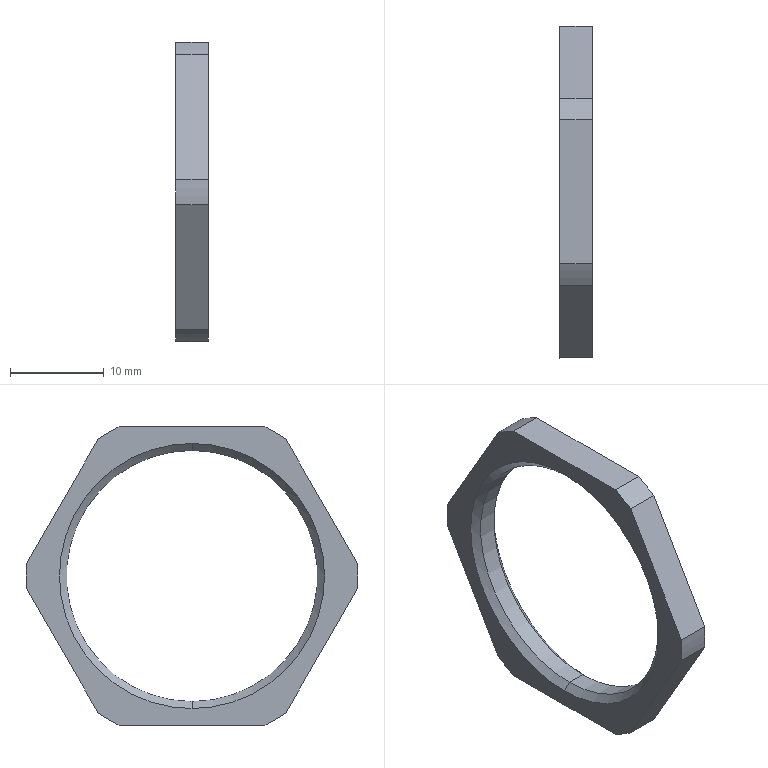Part | STEP file | 00373407_MUTTER_M_PG_21_DIN_46320-MS | 1 solid | 20 faces | box 3.5 x 35.5 x 32 mm | volume 1055 mm3 | cylinder 8 | plane 8 | cone 4 | commonest cylinder face diameters 35.5 x6 26.84 x2
STEP:
#1=CARTESIAN_POINT('',(0.,0.,0.));
#2=DIRECTION('',(0.,0.,1.));
#3=DIRECTION('',(1.,0.,0.));
#4=AXIS2_PLACEMENT_3D('',#1,#2,#3);
#5=CARTESIAN_POINT('',(2.75,0.,-13.42));
#6=VERTEX_POINT('',#5);
#7=CARTESIAN_POINT('',(3.5,0.,-14.17));
#8=VERTEX_POINT('',#7);
#9=CARTESIAN_POINT('',(3.5,0.,-14.17));
#10=DIRECTION('',(0.7071,0.,-0.7071));
#11=VECTOR('',#10,1.);
#12=LINE('',#9,#11);
#13=CARTESIAN_POINT('',(3.5,0.,0.));
#14=DIRECTION('',(1.,0.,0.));
#15=DIRECTION('',(0.,0.,-1.));
#16=AXIS2_PLACEMENT_3D('',#13,#14,#15);
#17=CONICAL_SURFACE('',#16,14.17,0.7854);
#18=CARTESIAN_POINT('',(6.283,0.));
#19=DIRECTION('',(0.,1.));
#20=VECTOR('',#19,1.);
#21=LINE('',#18,#20);
#22=(GEOMETRIC_REPRESENTATION_CONTEXT(2)PARAMETRIC_REPRESENTATION_CONTEXT()REPRESENTATION_CONTEXT('',''));
#23=DEFINITIONAL_REPRESENTATION('',(#21),#22);
#24=PCURVE('',#17,#23);
#25=CARTESIAN_POINT('',(3.5,0.,0.));
#26=DIRECTION('',(1.,0.,0.));
#27=DIRECTION('',(0.,0.,-1.));
#28=AXIS2_PLACEMENT_3D('',#25,#26,#27);
#29=CONICAL_SURFACE('',#28,14.17,0.7854);
#30=CARTESIAN_POINT('',(0.,0.));
#31=DIRECTION('',(0.,1.));
#32=VECTOR('',#31,1.);
#33=LINE('',#30,#32);
#34=(GEOMETRIC_REPRESENTATION_CONTEXT(2)PARAMETRIC_REPRESENTATION_CONTEXT()REPRESENTATION_CONTEXT('',''));
#35=DEFINITIONAL_REPRESENTATION('',(#33),#34);
#36=PCURVE('',#29,#35);
#37=SURFACE_CURVE('',#12,(#24,#36),.PCURVE_S1.);
#38=EDGE_CURVE('',#6,#8,#37,.T.);
#39=ORIENTED_EDGE('',*,*,#38,.T.);
#40=CARTESIAN_POINT('',(3.5,0.,14.17));
#41=VERTEX_POINT('',#40);
#42=CARTESIAN_POINT('',(3.5,0.,0.));
#43=DIRECTION('',(-1.,0.,0.));
#44=DIRECTION('',(0.,0.,-1.));
#45=AXIS2_PLACEMENT_3D('',#42,#43,#44);
#46=CIRCLE('',#45,14.17);
#47=CARTESIAN_POINT('',(6.283,0.));
#48=DIRECTION('',(-1.,0.));
#49=VECTOR('',#48,1.);
#50=LINE('',#47,#49);
#51=(GEOMETRIC_REPRESENTATION_CONTEXT(2)PARAMETRIC_REPRESENTATION_CONTEXT()REPRESENTATION_CONTEXT('',''));
#52=DEFINITIONAL_REPRESENTATION('',(#50),#51);
#53=PCURVE('',#17,#52);
#54=CARTESIAN_POINT('',(3.5,0.,0.));
#55=DIRECTION('',(1.,0.,0.));
#56=DIRECTION('',(0.,0.,-1.));
#57=AXIS2_PLACEMENT_3D('',#54,#55,#56);
#58=PLANE('',#57);
#59=CARTESIAN_POINT('',(14.17,0.));
#60=CARTESIAN_POINT('',(14.17,-24.543));
#61=CARTESIAN_POINT('',(-7.085,-12.272));
#62=CARTESIAN_POINT('',(-28.34,0.));
#63=CARTESIAN_POINT('',(-7.085,12.272));
#64=CARTESIAN_POINT('',(14.17,24.543));
#65=CARTESIAN_POINT('',(14.17,0.));
#66=(BOUNDED_CURVE()B_SPLINE_CURVE(2,(#59,#60,#61,#62,#63,#64,#65),.UNSPECIFIED.,.T.,.F.)B_SPLINE_CURVE_WITH_KNOTS((1,2,2,2,2,1),(-2.094,0.,2.094,4.189,6.283,8.378),.UNSPECIFIED.)CURVE()GEOMETRIC_REPRESENTATION_ITEM()RATIONAL_B_SPLINE_CURVE((1.,0.5,1.,0.5,1.,0.5,1.))REPRESENTATION_ITEM(''));
#67=(GEOMETRIC_REPRESENTATION_CONTEXT(2)PARAMETRIC_REPRESENTATION_CONTEXT()REPRESENTATION_CONTEXT('',''));
#68=DEFINITIONAL_REPRESENTATION('',(#66),#67);
#69=PCURVE('',#58,#68);
#70=SURFACE_CURVE('',#46,(#53,#69),.PCURVE_S1.);
#71=EDGE_CURVE('',#8,#41,#70,.T.);
#72=ORIENTED_EDGE('',*,*,#71,.T.);
#73=CARTESIAN_POINT('',(2.75,0.,13.42));
#74=VERTEX_POINT('',#73);
#75=CARTESIAN_POINT('',(3.5,0.,14.17));
#76=DIRECTION('',(0.7071,0.,0.7071));
#77=VECTOR('',#76,1.);
#78=LINE('',#75,#77);
#79=CARTESIAN_POINT('',(3.142,0.));
#80=DIRECTION('',(0.,1.));
#81=VECTOR('',#80,1.);
#82=LINE('',#79,#81);
#83=(GEOMETRIC_REPRESENTATION_CONTEXT(2)PARAMETRIC_REPRESENTATION_CONTEXT()REPRESENTATION_CONTEXT('',''));
#84=DEFINITIONAL_REPRESENTATION('',(#82),#83);
#85=PCURVE('',#17,#84);
#86=CARTESIAN_POINT('',(3.142,0.));
#87=DIRECTION('',(0.,1.));
#88=VECTOR('',#87,1.);
#89=LINE('',#86,#88);
#90=(GEOMETRIC_REPRESENTATION_CONTEXT(2)PARAMETRIC_REPRESENTATION_CONTEXT()REPRESENTATION_CONTEXT('',''));
#91=DEFINITIONAL_REPRESENTATION('',(#89),#90);
#92=PCURVE('',#29,#91);
#93=SURFACE_CURVE('',#78,(#85,#92),.PCURVE_S1.);
#94=EDGE_CURVE('',#74,#41,#93,.T.);
#95=ORIENTED_EDGE('',*,*,#94,.F.);
#96=CARTESIAN_POINT('',(2.75,0.,0.));
#97=DIRECTION('',(1.,0.,0.));
#98=DIRECTION('',(0.,-1.,0.));
#99=AXIS2_PLACEMENT_3D('',#96,#97,#98);
#100=CIRCLE('',#99,13.42);
#101=CARTESIAN_POINT('',(-1.571,-0.75));
#102=DIRECTION('',(1.,0.));
#103=VECTOR('',#102,1.);
#104=LINE('',#101,#103);
#105=(GEOMETRIC_REPRESENTATION_CONTEXT(2)PARAMETRIC_REPRESENTATION_CONTEXT()REPRESENTATION_CONTEXT('',''));
#106=DEFINITIONAL_REPRESENTATION('',(#104),#105);
#107=PCURVE('',#17,#106);
#108=CARTESIAN_POINT('',(11.,0.,0.));
#109=DIRECTION('',(1.,0.,0.));
#110=DIRECTION('',(0.,0.,-1.));
#111=AXIS2_PLACEMENT_3D('',#108,#109,#110);
#112=CYLINDRICAL_SURFACE('',#111,13.42);
#113=CARTESIAN_POINT('',(-1.571,-8.25));
#114=DIRECTION('',(1.,0.));
#115=VECTOR('',#114,1.);
#116=LINE('',#113,#115);
#117=(GEOMETRIC_REPRESENTATION_CONTEXT(2)PARAMETRIC_REPRESENTATION_CONTEXT()REPRESENTATION_CONTEXT('',''));
#118=DEFINITIONAL_REPRESENTATION('',(#116),#117);
#119=PCURVE('',#112,#118);
#120=SURFACE_CURVE('',#100,(#107,#119),.PCURVE_S1.);
#121=EDGE_CURVE('',#74,#6,#120,.T.);
#122=ORIENTED_EDGE('',*,*,#121,.T.);
#123=EDGE_LOOP('',(#39,#72,#95,#122));
#124=FACE_BOUND('',#123,.F.);
#125=ADVANCED_FACE('',(#124),#17,.F.);
#126=CARTESIAN_POINT('',(0.75,0.,-13.42));
#127=VERTEX_POINT('',#126);
#128=CARTESIAN_POINT('',(11.,0.,-13.42));
#129=DIRECTION('',(1.,0.,0.));
#130=VECTOR('',#129,1.);
#131=LINE('',#128,#130);
#132=CARTESIAN_POINT('',(6.283,0.));
#133=DIRECTION('',(0.,1.));
#134=VECTOR('',#133,1.);
#135=LINE('',#132,#134);
#136=(GEOMETRIC_REPRESENTATION_CONTEXT(2)PARAMETRIC_REPRESENTATION_CONTEXT()REPRESENTATION_CONTEXT('',''));
#137=DEFINITIONAL_REPRESENTATION('',(#135),#136);
#138=PCURVE('',#112,#137);
#139=CARTESIAN_POINT('',(11.,0.,0.));
#140=DIRECTION('',(1.,0.,0.));
#141=DIRECTION('',(0.,0.,-1.));
#142=AXIS2_PLACEMENT_3D('',#139,#140,#141);
#143=CYLINDRICAL_SURFACE('',#142,13.42);
#144=CARTESIAN_POINT('',(0.,0.));
#145=DIRECTION('',(0.,1.));
#146=VECTOR('',#145,1.);
#147=LINE('',#144,#146);
#148=(GEOMETRIC_REPRESENTATION_CONTEXT(2)PARAMETRIC_REPRESENTATION_CONTEXT()REPRESENTATION_CONTEXT('',''));
#149=DEFINITIONAL_REPRESENTATION('',(#147),#148);
#150=PCURVE('',#143,#149);
#151=SURFACE_CURVE('',#131,(#138,#150),.PCURVE_S1.);
#152=EDGE_CURVE('',#127,#6,#151,.T.);
#153=ORIENTED_EDGE('',*,*,#152,.T.);
#154=ORIENTED_EDGE('',*,*,#121,.F.);
#155=CARTESIAN_POINT('',(0.75,0.,13.42));
#156=VERTEX_POINT('',#155);
#157=CARTESIAN_POINT('',(11.,0.,13.42));
#158=DIRECTION('',(1.,0.,0.));
#159=VECTOR('',#158,1.);
#160=LINE('',#157,#159);
#161=CARTESIAN_POINT('',(3.142,0.));
#162=DIRECTION('',(0.,1.));
#163=VECTOR('',#162,1.);
#164=LINE('',#161,#163);
#165=(GEOMETRIC_REPRESENTATION_CONTEXT(2)PARAMETRIC_REPRESENTATION_CONTEXT()REPRESENTATION_CONTEXT('',''));
#166=DEFINITIONAL_REPRESENTATION('',(#164),#165);
#167=PCURVE('',#112,#166);
#168=CARTESIAN_POINT('',(3.142,0.));
#169=DIRECTION('',(0.,1.));
#170=VECTOR('',#169,1.);
#171=LINE('',#168,#170);
#172=(GEOMETRIC_REPRESENTATION_CONTEXT(2)PARAMETRIC_REPRESENTATION_CONTEXT()REPRESENTATION_CONTEXT('',''));
#173=DEFINITIONAL_REPRESENTATION('',(#171),#172);
#174=PCURVE('',#143,#173);
#175=SURFACE_CURVE('',#160,(#167,#174),.PCURVE_S1.);
#176=EDGE_CURVE('',#156,#74,#175,.T.);
#177=ORIENTED_EDGE('',*,*,#176,.F.);
#178=CARTESIAN_POINT('',(0.75,0.,0.));
#179=DIRECTION('',(1.,0.,0.));
#180=DIRECTION('',(0.,0.,-1.));
#181=AXIS2_PLACEMENT_3D('',#178,#179,#180);
#182=CIRCLE('',#181,13.42);
#183=CARTESIAN_POINT('',(0.,-10.25));
#184=DIRECTION('',(1.,0.));
#185=VECTOR('',#184,1.);
#186=LINE('',#183,#185);
#187=(GEOMETRIC_REPRESENTATION_CONTEXT(2)PARAMETRIC_REPRESENTATION_CONTEXT()REPRESENTATION_CONTEXT('',''));
#188=DEFINITIONAL_REPRESENTATION('',(#186),#187);
#189=PCURVE('',#112,#188);
#190=CARTESIAN_POINT('',(0.,0.,0.));
#191=DIRECTION('',(-1.,0.,0.));
#192=DIRECTION('',(0.,0.,1.));
#193=AXIS2_PLACEMENT_3D('',#190,#191,#192);
#194=CONICAL_SURFACE('',#193,14.17,0.7854);
#195=CARTESIAN_POINT('',(9.425,-0.75));
#196=DIRECTION('',(-1.,0.));
#197=VECTOR('',#196,1.);
#198=LINE('',#195,#197);
#199=(GEOMETRIC_REPRESENTATION_CONTEXT(2)PARAMETRIC_REPRESENTATION_CONTEXT()REPRESENTATION_CONTEXT('',''));
#200=DEFINITIONAL_REPRESENTATION('',(#198),#199);
#201=PCURVE('',#194,#200);
#202=SURFACE_CURVE('',#182,(#189,#201),.PCURVE_S1.);
#203=EDGE_CURVE('',#156,#127,#202,.T.);
#204=ORIENTED_EDGE('',*,*,#203,.T.);
#205=EDGE_LOOP('',(#153,#154,#177,#204));
#206=FACE_BOUND('',#205,.F.);
#207=ADVANCED_FACE('',(#206),#112,.F.);
#208=CARTESIAN_POINT('',(0.,0.,14.17));
#209=VERTEX_POINT('',#208);
#210=CARTESIAN_POINT('',(0.,0.,14.17));
#211=DIRECTION('',(-0.7071,0.,0.7071));
#212=VECTOR('',#211,1.);
#213=LINE('',#210,#212);
#214=CARTESIAN_POINT('',(6.283,0.));
#215=DIRECTION('',(0.,1.));
#216=VECTOR('',#215,1.);
#217=LINE('',#214,#216);
#218=(GEOMETRIC_REPRESENTATION_CONTEXT(2)PARAMETRIC_REPRESENTATION_CONTEXT()REPRESENTATION_CONTEXT('',''));
#219=DEFINITIONAL_REPRESENTATION('',(#217),#218);
#220=PCURVE('',#194,#219);
#221=CARTESIAN_POINT('',(0.,0.,0.));
#222=DIRECTION('',(-1.,0.,0.));
#223=DIRECTION('',(0.,0.,1.));
#224=AXIS2_PLACEMENT_3D('',#221,#222,#223);
#225=CONICAL_SURFACE('',#224,14.17,0.7854);
#226=CARTESIAN_POINT('',(0.,0.));
#227=DIRECTION('',(0.,1.));
#228=VECTOR('',#227,1.);
#229=LINE('',#226,#228);
#230=(GEOMETRIC_REPRESENTATION_CONTEXT(2)PARAMETRIC_REPRESENTATION_CONTEXT()REPRESENTATION_CONTEXT('',''));
#231=DEFINITIONAL_REPRESENTATION('',(#229),#230);
#232=PCURVE('',#225,#231);
#233=SURFACE_CURVE('',#213,(#220,#232),.PCURVE_S1.);
#234=EDGE_CURVE('',#156,#209,#233,.T.);
#235=ORIENTED_EDGE('',*,*,#234,.T.);
#236=CARTESIAN_POINT('',(0.,0.,-14.17));
#237=VERTEX_POINT('',#236);
#238=CARTESIAN_POINT('',(0.,0.,0.));
#239=DIRECTION('',(-1.,0.,0.));
#240=DIRECTION('',(0.,0.,1.));
#241=AXIS2_PLACEMENT_3D('',#238,#239,#240);
#242=CIRCLE('',#241,14.17);
#243=CARTESIAN_POINT('',(0.,0.));
#244=DIRECTION('',(1.,0.));
#245=VECTOR('',#244,1.);
#246=LINE('',#243,#245);
#247=(GEOMETRIC_REPRESENTATION_CONTEXT(2)PARAMETRIC_REPRESENTATION_CONTEXT()REPRESENTATION_CONTEXT('',''));
#248=DEFINITIONAL_REPRESENTATION('',(#246),#247);
#249=PCURVE('',#194,#248);
#250=CARTESIAN_POINT('',(0.,0.,0.));
#251=DIRECTION('',(1.,0.,0.));
#252=DIRECTION('',(0.,0.,-1.));
#253=AXIS2_PLACEMENT_3D('',#250,#251,#252);
#254=PLANE('',#253);
#255=CARTESIAN_POINT('',(-14.17,0.));
#256=CARTESIAN_POINT('',(-14.17,24.543));
#257=CARTESIAN_POINT('',(7.085,12.272));
#258=CARTESIAN_POINT('',(28.34,0.));
#259=CARTESIAN_POINT('',(7.085,-12.272));
#260=CARTESIAN_POINT('',(-14.17,-24.543));
#261=CARTESIAN_POINT('',(-14.17,0.));
#262=(BOUNDED_CURVE()B_SPLINE_CURVE(2,(#255,#256,#257,#258,#259,#260,#261),.UNSPECIFIED.,.T.,.F.)B_SPLINE_CURVE_WITH_KNOTS((1,2,2,2,2,1),(-2.094,0.,2.094,4.189,6.283,8.378),.UNSPECIFIED.)CURVE()GEOMETRIC_REPRESENTATION_ITEM()RATIONAL_B_SPLINE_CURVE((1.,0.5,1.,0.5,1.,0.5,1.))REPRESENTATION_ITEM(''));
#263=(GEOMETRIC_REPRESENTATION_CONTEXT(2)PARAMETRIC_REPRESENTATION_CONTEXT()REPRESENTATION_CONTEXT('',''));
#264=DEFINITIONAL_REPRESENTATION('',(#262),#263);
#265=PCURVE('',#254,#264);
#266=SURFACE_CURVE('',#242,(#249,#265),.PCURVE_S1.);
#267=EDGE_CURVE('',#237,#209,#266,.T.);
#268=ORIENTED_EDGE('',*,*,#267,.F.);
#269=CARTESIAN_POINT('',(0.,0.,-14.17));
#270=DIRECTION('',(-0.7071,0.,-0.7071));
#271=VECTOR('',#270,1.);
#272=LINE('',#269,#271);
#273=CARTESIAN_POINT('',(3.142,0.));
#274=DIRECTION('',(0.,1.));
#275=VECTOR('',#274,1.);
#276=LINE('',#273,#275);
#277=(GEOMETRIC_REPRESENTATION_CONTEXT(2)PARAMETRIC_REPRESENTATION_CONTEXT()REPRESENTATION_CONTEXT('',''));
#278=DEFINITIONAL_REPRESENTATION('',(#276),#277);
#279=PCURVE('',#194,#278);
#280=CARTESIAN_POINT('',(3.142,0.));
#281=DIRECTION('',(0.,1.));
#282=VECTOR('',#281,1.);
#283=LINE('',#280,#282);
#284=(GEOMETRIC_REPRESENTATION_CONTEXT(2)PARAMETRIC_REPRESENTATION_CONTEXT()REPRESENTATION_CONTEXT('',''));
#285=DEFINITIONAL_REPRESENTATION('',(#283),#284);
#286=PCURVE('',#225,#285);
#287=SURFACE_CURVE('',#272,(#279,#286),.PCURVE_S1.);
#288=EDGE_CURVE('',#127,#237,#287,.T.);
#289=ORIENTED_EDGE('',*,*,#288,.F.);
#290=ORIENTED_EDGE('',*,*,#203,.F.);
#291=EDGE_LOOP('',(#235,#268,#289,#290));
#292=FACE_BOUND('',#291,.F.);
#293=ADVANCED_FACE('',(#292),#194,.F.);
#294=CARTESIAN_POINT('',(0.,0.,0.));
#295=DIRECTION('',(-1.,0.,0.));
#296=DIRECTION('',(0.,0.,1.));
#297=AXIS2_PLACEMENT_3D('',#294,#295,#296);
#298=CIRCLE('',#297,14.17);
#299=CARTESIAN_POINT('',(0.,0.));
#300=DIRECTION('',(1.,0.));
#301=VECTOR('',#300,1.);
#302=LINE('',#299,#301);
#303=(GEOMETRIC_REPRESENTATION_CONTEXT(2)PARAMETRIC_REPRESENTATION_CONTEXT()REPRESENTATION_CONTEXT('',''));
#304=DEFINITIONAL_REPRESENTATION('',(#302),#303);
#305=PCURVE('',#225,#304);
#306=CARTESIAN_POINT('',(-14.17,0.));
#307=CARTESIAN_POINT('',(-14.17,24.543));
#308=CARTESIAN_POINT('',(7.085,12.272));
#309=CARTESIAN_POINT('',(28.34,0.));
#310=CARTESIAN_POINT('',(7.085,-12.272));
#311=CARTESIAN_POINT('',(-14.17,-24.543));
#312=CARTESIAN_POINT('',(-14.17,0.));
#313=(BOUNDED_CURVE()B_SPLINE_CURVE(2,(#306,#307,#308,#309,#310,#311,#312),.UNSPECIFIED.,.T.,.F.)B_SPLINE_CURVE_WITH_KNOTS((1,2,2,2,2,1),(-2.094,0.,2.094,4.189,6.283,8.378),.UNSPECIFIED.)CURVE()GEOMETRIC_REPRESENTATION_ITEM()RATIONAL_B_SPLINE_CURVE((1.,0.5,1.,0.5,1.,0.5,1.))REPRESENTATION_ITEM(''));
#314=(GEOMETRIC_REPRESENTATION_CONTEXT(2)PARAMETRIC_REPRESENTATION_CONTEXT()REPRESENTATION_CONTEXT('',''));
#315=DEFINITIONAL_REPRESENTATION('',(#313),#314);
#316=PCURVE('',#254,#315);
#317=SURFACE_CURVE('',#298,(#305,#316),.PCURVE_S1.);
#318=EDGE_CURVE('',#209,#237,#317,.T.);
#319=ORIENTED_EDGE('',*,*,#318,.F.);
#320=ORIENTED_EDGE('',*,*,#234,.F.);
#321=CARTESIAN_POINT('',(0.75,0.,0.));
#322=DIRECTION('',(1.,0.,0.));
#323=DIRECTION('',(0.,0.,-1.));
#324=AXIS2_PLACEMENT_3D('',#321,#322,#323);
#325=CIRCLE('',#324,13.42);
#326=CARTESIAN_POINT('',(3.142,-0.75));
#327=DIRECTION('',(-1.,0.));
#328=VECTOR('',#327,1.);
#329=LINE('',#326,#328);
#330=(GEOMETRIC_REPRESENTATION_CONTEXT(2)PARAMETRIC_REPRESENTATION_CONTEXT()REPRESENTATION_CONTEXT('',''));
#331=DEFINITIONAL_REPRESENTATION('',(#329),#330);
#332=PCURVE('',#225,#331);
#333=CARTESIAN_POINT('',(0.,-10.25));
#334=DIRECTION('',(1.,0.));
#335=VECTOR('',#334,1.);
#336=LINE('',#333,#335);
#337=(GEOMETRIC_REPRESENTATION_CONTEXT(2)PARAMETRIC_REPRESENTATION_CONTEXT()REPRESENTATION_CONTEXT('',''));
#338=DEFINITIONAL_REPRESENTATION('',(#336),#337);
#339=PCURVE('',#143,#338);
#340=SURFACE_CURVE('',#325,(#332,#339),.PCURVE_S1.);
#341=EDGE_CURVE('',#127,#156,#340,.T.);
#342=ORIENTED_EDGE('',*,*,#341,.F.);
#343=ORIENTED_EDGE('',*,*,#288,.T.);
#344=EDGE_LOOP('',(#319,#320,#342,#343));
#345=FACE_BOUND('',#344,.F.);
#346=ADVANCED_FACE('',(#345),#225,.F.);
#347=CARTESIAN_POINT('',(3.5,17.699,1.344));
#348=VERTEX_POINT('',#347);
#349=CARTESIAN_POINT('',(3.5,17.699,-1.344));
#350=VERTEX_POINT('',#349);
#351=CARTESIAN_POINT('',(3.5,0.,0.));
#352=DIRECTION('',(-1.,0.,0.));
#353=DIRECTION('',(0.,0.,-1.));
#354=AXIS2_PLACEMENT_3D('',#351,#352,#353);
#355=CIRCLE('',#354,17.75);
#356=CARTESIAN_POINT('',(11.,0.,0.));
#357=DIRECTION('',(1.,0.,0.));
#358=DIRECTION('',(0.,0.,-1.));
#359=AXIS2_PLACEMENT_3D('',#356,#357,#358);
#360=CYLINDRICAL_SURFACE('',#359,17.75);
#361=CARTESIAN_POINT('',(6.283,-7.5));
#362=DIRECTION('',(-1.,0.));
#363=VECTOR('',#362,1.);
#364=LINE('',#361,#363);
#365=(GEOMETRIC_REPRESENTATION_CONTEXT(2)PARAMETRIC_REPRESENTATION_CONTEXT()REPRESENTATION_CONTEXT('',''));
#366=DEFINITIONAL_REPRESENTATION('',(#364),#365);
#367=PCURVE('',#360,#366);
#368=CARTESIAN_POINT('',(17.75,0.));
#369=CARTESIAN_POINT('',(17.75,-30.744));
#370=CARTESIAN_POINT('',(-8.875,-15.372));
#371=CARTESIAN_POINT('',(-35.5,0.));
#372=CARTESIAN_POINT('',(-8.875,15.372));
#373=CARTESIAN_POINT('',(17.75,30.744));
#374=CARTESIAN_POINT('',(17.75,0.));
#375=(BOUNDED_CURVE()B_SPLINE_CURVE(2,(#368,#369,#370,#371,#372,#373,#374),.UNSPECIFIED.,.T.,.F.)B_SPLINE_CURVE_WITH_KNOTS((1,2,2,2,2,1),(-2.094,0.,2.094,4.189,6.283,8.378),.UNSPECIFIED.)CURVE()GEOMETRIC_REPRESENTATION_ITEM()RATIONAL_B_SPLINE_CURVE((1.,0.5,1.,0.5,1.,0.5,1.))REPRESENTATION_ITEM(''));
#376=(GEOMETRIC_REPRESENTATION_CONTEXT(2)PARAMETRIC_REPRESENTATION_CONTEXT()REPRESENTATION_CONTEXT('',''));
#377=DEFINITIONAL_REPRESENTATION('',(#375),#376);
#378=PCURVE('',#58,#377);
#379=SURFACE_CURVE('',#355,(#367,#378),.PCURVE_S1.);
#380=EDGE_CURVE('',#348,#350,#379,.T.);
#381=ORIENTED_EDGE('',*,*,#380,.T.);
#382=CARTESIAN_POINT('',(0.,17.699,-1.344));
#383=VERTEX_POINT('',#382);
#384=CARTESIAN_POINT('',(0.5,17.699,-1.344));
#385=DIRECTION('',(-1.,0.,0.));
#386=VECTOR('',#385,1.);
#387=LINE('',#384,#386);
#388=CARTESIAN_POINT('',(1.495,-10.5));
#389=DIRECTION('',(0.,-1.));
#390=VECTOR('',#389,1.);
#391=LINE('',#388,#390);
#392=(GEOMETRIC_REPRESENTATION_CONTEXT(2)PARAMETRIC_REPRESENTATION_CONTEXT()REPRESENTATION_CONTEXT('',''));
#393=DEFINITIONAL_REPRESENTATION('',(#391),#392);
#394=PCURVE('',#360,#393);
#395=CARTESIAN_POINT('',(0.5,13.856,-8.));
#396=DIRECTION('',(0.,-0.866,0.5));
#397=DIRECTION('',(0.,-0.5,-0.866));
#398=AXIS2_PLACEMENT_3D('',#395,#396,#397);
#399=PLANE('',#398);
#400=CARTESIAN_POINT('',(-7.685,0.));
#401=DIRECTION('',(0.,-1.));
#402=VECTOR('',#401,1.);
#403=LINE('',#400,#402);
#404=(GEOMETRIC_REPRESENTATION_CONTEXT(2)PARAMETRIC_REPRESENTATION_CONTEXT()REPRESENTATION_CONTEXT('',''));
#405=DEFINITIONAL_REPRESENTATION('',(#403),#404);
#406=PCURVE('',#399,#405);
#407=SURFACE_CURVE('',#387,(#394,#406),.PCURVE_S1.);
#408=EDGE_CURVE('',#350,#383,#407,.T.);
#409=ORIENTED_EDGE('',*,*,#408,.T.);
#410=CARTESIAN_POINT('',(0.,17.699,1.344));
#411=VERTEX_POINT('',#410);
#412=CARTESIAN_POINT('',(0.,0.,0.));
#413=DIRECTION('',(1.,0.,0.));
#414=DIRECTION('',(0.,0.,-1.));
#415=AXIS2_PLACEMENT_3D('',#412,#413,#414);
#416=CIRCLE('',#415,17.75);
#417=CARTESIAN_POINT('',(0.,-11.));
#418=DIRECTION('',(1.,0.));
#419=VECTOR('',#418,1.);
#420=LINE('',#417,#419);
#421=(GEOMETRIC_REPRESENTATION_CONTEXT(2)PARAMETRIC_REPRESENTATION_CONTEXT()REPRESENTATION_CONTEXT('',''));
#422=DEFINITIONAL_REPRESENTATION('',(#420),#421);
#423=PCURVE('',#360,#422);
#424=CARTESIAN_POINT('',(0.,0.));
#425=DIRECTION('',(1.,0.));
#426=AXIS2_PLACEMENT_2D('',#424,#425);
#427=CIRCLE('',#426,17.75);
#428=(GEOMETRIC_REPRESENTATION_CONTEXT(2)PARAMETRIC_REPRESENTATION_CONTEXT()REPRESENTATION_CONTEXT('',''));
#429=DEFINITIONAL_REPRESENTATION('',(#427),#428);
#430=PCURVE('',#254,#429);
#431=SURFACE_CURVE('',#416,(#423,#430),.PCURVE_S1.);
#432=EDGE_CURVE('',#383,#411,#431,.T.);
#433=ORIENTED_EDGE('',*,*,#432,.T.);
#434=CARTESIAN_POINT('',(0.5,17.699,1.344));
#435=DIRECTION('',(1.,0.,0.));
#436=VECTOR('',#435,1.);
#437=LINE('',#434,#436);
#438=CARTESIAN_POINT('',(1.647,-10.5));
#439=DIRECTION('',(0.,1.));
#440=VECTOR('',#439,1.);
#441=LINE('',#438,#440);
#442=(GEOMETRIC_REPRESENTATION_CONTEXT(2)PARAMETRIC_REPRESENTATION_CONTEXT()REPRESENTATION_CONTEXT('',''));
#443=DEFINITIONAL_REPRESENTATION('',(#441),#442);
#444=PCURVE('',#360,#443);
#445=CARTESIAN_POINT('',(0.5,13.856,8.));
#446=DIRECTION('',(0.,-0.866,-0.5));
#447=DIRECTION('',(0.,0.5,-0.866));
#448=AXIS2_PLACEMENT_3D('',#445,#446,#447);
#449=PLANE('',#448);
#450=CARTESIAN_POINT('',(7.685,0.));
#451=DIRECTION('',(0.,1.));
#452=VECTOR('',#451,1.);
#453=LINE('',#450,#452);
#454=(GEOMETRIC_REPRESENTATION_CONTEXT(2)PARAMETRIC_REPRESENTATION_CONTEXT()REPRESENTATION_CONTEXT('',''));
#455=DEFINITIONAL_REPRESENTATION('',(#453),#454);
#456=PCURVE('',#449,#455);
#457=SURFACE_CURVE('',#437,(#444,#456),.PCURVE_S1.);
#458=EDGE_CURVE('',#411,#348,#457,.T.);
#459=ORIENTED_EDGE('',*,*,#458,.T.);
#460=EDGE_LOOP('',(#381,#409,#433,#459));
#461=FACE_BOUND('',#460,.T.);
#462=ADVANCED_FACE('',(#461),#360,.T.);
#463=CARTESIAN_POINT('',(0.,-17.699,-1.344));
#464=VERTEX_POINT('',#463);
#465=CARTESIAN_POINT('',(3.5,-17.699,-1.344));
#466=VERTEX_POINT('',#465);
#467=CARTESIAN_POINT('',(0.5,-17.699,-1.344));
#468=DIRECTION('',(1.,0.,0.));
#469=VECTOR('',#468,1.);
#470=LINE('',#467,#469);
#471=CARTESIAN_POINT('',(11.,0.,0.));
#472=DIRECTION('',(1.,0.,0.));
#473=DIRECTION('',(0.,0.,-1.));
#474=AXIS2_PLACEMENT_3D('',#471,#472,#473);
#475=CYLINDRICAL_SURFACE('',#474,17.75);
#476=CARTESIAN_POINT('',(4.788,-10.5));
#477=DIRECTION('',(0.,1.));
#478=VECTOR('',#477,1.);
#479=LINE('',#476,#478);
#480=(GEOMETRIC_REPRESENTATION_CONTEXT(2)PARAMETRIC_REPRESENTATION_CONTEXT()REPRESENTATION_CONTEXT('',''));
#481=DEFINITIONAL_REPRESENTATION('',(#479),#480);
#482=PCURVE('',#475,#481);
#483=CARTESIAN_POINT('',(0.5,-13.856,-8.));
#484=DIRECTION('',(0.,0.866,0.5));
#485=DIRECTION('',(0.,-0.5,0.866));
#486=AXIS2_PLACEMENT_3D('',#483,#484,#485);
#487=PLANE('',#486);
#488=CARTESIAN_POINT('',(7.685,0.));
#489=DIRECTION('',(0.,1.));
#490=VECTOR('',#489,1.);
#491=LINE('',#488,#490);
#492=(GEOMETRIC_REPRESENTATION_CONTEXT(2)PARAMETRIC_REPRESENTATION_CONTEXT()REPRESENTATION_CONTEXT('',''));
#493=DEFINITIONAL_REPRESENTATION('',(#491),#492);
#494=PCURVE('',#487,#493);
#495=SURFACE_CURVE('',#470,(#482,#494),.PCURVE_S1.);
#496=EDGE_CURVE('',#464,#466,#495,.T.);
#497=ORIENTED_EDGE('',*,*,#496,.T.);
#498=CARTESIAN_POINT('',(3.5,-17.699,1.344));
#499=VERTEX_POINT('',#498);
#500=CARTESIAN_POINT('',(3.5,0.,0.));
#501=DIRECTION('',(-1.,0.,0.));
#502=DIRECTION('',(0.,0.,-1.));
#503=AXIS2_PLACEMENT_3D('',#500,#501,#502);
#504=CIRCLE('',#503,17.75);
#505=CARTESIAN_POINT('',(6.283,-7.5));
#506=DIRECTION('',(-1.,0.));
#507=VECTOR('',#506,1.);
#508=LINE('',#505,#507);
#509=(GEOMETRIC_REPRESENTATION_CONTEXT(2)PARAMETRIC_REPRESENTATION_CONTEXT()REPRESENTATION_CONTEXT('',''));
#510=DEFINITIONAL_REPRESENTATION('',(#508),#509);
#511=PCURVE('',#475,#510);
#512=CARTESIAN_POINT('',(17.75,0.));
#513=CARTESIAN_POINT('',(17.75,-30.744));
#514=CARTESIAN_POINT('',(-8.875,-15.372));
#515=CARTESIAN_POINT('',(-35.5,0.));
#516=CARTESIAN_POINT('',(-8.875,15.372));
#517=CARTESIAN_POINT('',(17.75,30.744));
#518=CARTESIAN_POINT('',(17.75,0.));
#519=(BOUNDED_CURVE()B_SPLINE_CURVE(2,(#512,#513,#514,#515,#516,#517,#518),.UNSPECIFIED.,.T.,.F.)B_SPLINE_CURVE_WITH_KNOTS((1,2,2,2,2,1),(-2.094,0.,2.094,4.189,6.283,8.378),.UNSPECIFIED.)CURVE()GEOMETRIC_REPRESENTATION_ITEM()RATIONAL_B_SPLINE_CURVE((1.,0.5,1.,0.5,1.,0.5,1.))REPRESENTATION_ITEM(''));
#520=(GEOMETRIC_REPRESENTATION_CONTEXT(2)PARAMETRIC_REPRESENTATION_CONTEXT()REPRESENTATION_CONTEXT('',''));
#521=DEFINITIONAL_REPRESENTATION('',(#519),#520);
#522=PCURVE('',#58,#521);
#523=SURFACE_CURVE('',#504,(#511,#522),.PCURVE_S1.);
#524=EDGE_CURVE('',#466,#499,#523,.T.);
#525=ORIENTED_EDGE('',*,*,#524,.T.);
#526=CARTESIAN_POINT('',(0.,-17.699,1.344));
#527=VERTEX_POINT('',#526);
#528=CARTESIAN_POINT('',(0.5,-17.699,1.344));
#529=DIRECTION('',(-1.,0.,0.));
#530=VECTOR('',#529,1.);
#531=LINE('',#528,#530);
#532=CARTESIAN_POINT('',(4.637,-10.5));
#533=DIRECTION('',(0.,-1.));
#534=VECTOR('',#533,1.);
#535=LINE('',#532,#534);
#536=(GEOMETRIC_REPRESENTATION_CONTEXT(2)PARAMETRIC_REPRESENTATION_CONTEXT()REPRESENTATION_CONTEXT('',''));
#537=DEFINITIONAL_REPRESENTATION('',(#535),#536);
#538=PCURVE('',#475,#537);
#539=CARTESIAN_POINT('',(0.5,-13.856,8.));
#540=DIRECTION('',(0.,0.866,-0.5));
#541=DIRECTION('',(0.,0.5,0.866));
#542=AXIS2_PLACEMENT_3D('',#539,#540,#541);
#543=PLANE('',#542);
#544=CARTESIAN_POINT('',(-7.685,0.));
#545=DIRECTION('',(0.,-1.));
#546=VECTOR('',#545,1.);
#547=LINE('',#544,#546);
#548=(GEOMETRIC_REPRESENTATION_CONTEXT(2)PARAMETRIC_REPRESENTATION_CONTEXT()REPRESENTATION_CONTEXT('',''));
#549=DEFINITIONAL_REPRESENTATION('',(#547),#548);
#550=PCURVE('',#543,#549);
#551=SURFACE_CURVE('',#531,(#538,#550),.PCURVE_S1.);
#552=EDGE_CURVE('',#499,#527,#551,.T.);
#553=ORIENTED_EDGE('',*,*,#552,.T.);
#554=CARTESIAN_POINT('',(0.,0.,0.));
#555=DIRECTION('',(1.,0.,0.));
#556=DIRECTION('',(0.,0.,-1.));
#557=AXIS2_PLACEMENT_3D('',#554,#555,#556);
#558=CIRCLE('',#557,17.75);
#559=CARTESIAN_POINT('',(0.,-11.));
#560=DIRECTION('',(1.,0.));
#561=VECTOR('',#560,1.);
#562=LINE('',#559,#561);
#563=(GEOMETRIC_REPRESENTATION_CONTEXT(2)PARAMETRIC_REPRESENTATION_CONTEXT()REPRESENTATION_CONTEXT('',''));
#564=DEFINITIONAL_REPRESENTATION('',(#562),#563);
#565=PCURVE('',#475,#564);
#566=CARTESIAN_POINT('',(0.,0.));
#567=DIRECTION('',(1.,0.));
#568=AXIS2_PLACEMENT_2D('',#566,#567);
#569=CIRCLE('',#568,17.75);
#570=(GEOMETRIC_REPRESENTATION_CONTEXT(2)PARAMETRIC_REPRESENTATION_CONTEXT()REPRESENTATION_CONTEXT('',''));
#571=DEFINITIONAL_REPRESENTATION('',(#569),#570);
#572=PCURVE('',#254,#571);
#573=SURFACE_CURVE('',#558,(#565,#572),.PCURVE_S1.);
#574=EDGE_CURVE('',#527,#464,#573,.T.);
#575=ORIENTED_EDGE('',*,*,#574,.T.);
#576=EDGE_LOOP('',(#497,#525,#553,#575));
#577=FACE_BOUND('',#576,.T.);
#578=ADVANCED_FACE('',(#577),#475,.T.);
#579=ORIENTED_EDGE('',*,*,#318,.F.);
#580=ORIENTED_EDGE('',*,*,#267,.F.);
#581=EDGE_LOOP('',(#579,#580));
#582=FACE_BOUND('',#581,.T.);
#583=CARTESIAN_POINT('',(0.,7.685,-16.));
#584=VERTEX_POINT('',#583);
#585=CARTESIAN_POINT('',(0.,-7.685,-16.));
#586=VERTEX_POINT('',#585);
#587=CARTESIAN_POINT('',(0.,0.,-16.));
#588=DIRECTION('',(0.,-1.,0.));
#589=VECTOR('',#588,1.);
#590=LINE('',#587,#589);
#591=CARTESIAN_POINT('',(16.,0.));
#592=DIRECTION('',(0.,-1.));
#593=VECTOR('',#592,1.);
#594=LINE('',#591,#593);
#595=(GEOMETRIC_REPRESENTATION_CONTEXT(2)PARAMETRIC_REPRESENTATION_CONTEXT()REPRESENTATION_CONTEXT('',''));
#596=DEFINITIONAL_REPRESENTATION('',(#594),#595);
#597=PCURVE('',#254,#596);
#598=CARTESIAN_POINT('',(0.5,0.,-16.));
#599=DIRECTION('',(0.,0.,1.));
#600=DIRECTION('',(1.,0.,0.));
#601=AXIS2_PLACEMENT_3D('',#598,#599,#600);
#602=PLANE('',#601);
#603=CARTESIAN_POINT('',(-0.5,0.));
#604=DIRECTION('',(0.,-1.));
#605=VECTOR('',#604,1.);
#606=LINE('',#603,#605);
#607=(GEOMETRIC_REPRESENTATION_CONTEXT(2)PARAMETRIC_REPRESENTATION_CONTEXT()REPRESENTATION_CONTEXT('',''));
#608=DEFINITIONAL_REPRESENTATION('',(#606),#607);
#609=PCURVE('',#602,#608);
#610=SURFACE_CURVE('',#590,(#597,#609),.PCURVE_S1.);
#611=EDGE_CURVE('',#584,#586,#610,.T.);
#612=ORIENTED_EDGE('',*,*,#611,.T.);
#613=CARTESIAN_POINT('',(0.,-10.014,-14.656));
#614=VERTEX_POINT('',#613);
#615=CARTESIAN_POINT('',(0.,0.,0.));
#616=DIRECTION('',(1.,0.,0.));
#617=DIRECTION('',(0.,0.,-1.));
#618=AXIS2_PLACEMENT_3D('',#615,#616,#617);
#619=CIRCLE('',#618,17.75);
#620=CARTESIAN_POINT('',(0.,0.));
#621=DIRECTION('',(1.,0.));
#622=AXIS2_PLACEMENT_2D('',#620,#621);
#623=CIRCLE('',#622,17.75);
#624=(GEOMETRIC_REPRESENTATION_CONTEXT(2)PARAMETRIC_REPRESENTATION_CONTEXT()REPRESENTATION_CONTEXT('',''));
#625=DEFINITIONAL_REPRESENTATION('',(#623),#624);
#626=PCURVE('',#254,#625);
#627=CARTESIAN_POINT('',(11.,0.,0.));
#628=DIRECTION('',(1.,0.,0.));
#629=DIRECTION('',(0.,0.,-1.));
#630=AXIS2_PLACEMENT_3D('',#627,#628,#629);
#631=CYLINDRICAL_SURFACE('',#630,17.75);
#632=CARTESIAN_POINT('',(0.,-11.));
#633=DIRECTION('',(1.,0.));
#634=VECTOR('',#633,1.);
#635=LINE('',#632,#634);
#636=(GEOMETRIC_REPRESENTATION_CONTEXT(2)PARAMETRIC_REPRESENTATION_CONTEXT()REPRESENTATION_CONTEXT('',''));
#637=DEFINITIONAL_REPRESENTATION('',(#635),#636);
#638=PCURVE('',#631,#637);
#639=SURFACE_CURVE('',#619,(#626,#638),.PCURVE_S1.);
#640=EDGE_CURVE('',#614,#586,#639,.T.);
#641=ORIENTED_EDGE('',*,*,#640,.F.);
#642=CARTESIAN_POINT('',(0.,-13.856,-8.));
#643=DIRECTION('',(0.,-0.5,0.866));
#644=VECTOR('',#643,1.);
#645=LINE('',#642,#644);
#646=CARTESIAN_POINT('',(8.,-13.856));
#647=DIRECTION('',(-0.866,-0.5));
#648=VECTOR('',#647,1.);
#649=LINE('',#646,#648);
#650=(GEOMETRIC_REPRESENTATION_CONTEXT(2)PARAMETRIC_REPRESENTATION_CONTEXT()REPRESENTATION_CONTEXT('',''));
#651=DEFINITIONAL_REPRESENTATION('',(#649),#650);
#652=PCURVE('',#254,#651);
#653=CARTESIAN_POINT('',(0.,-0.5));
#654=DIRECTION('',(1.,0.));
#655=VECTOR('',#654,1.);
#656=LINE('',#653,#655);
#657=(GEOMETRIC_REPRESENTATION_CONTEXT(2)PARAMETRIC_REPRESENTATION_CONTEXT()REPRESENTATION_CONTEXT('',''));
#658=DEFINITIONAL_REPRESENTATION('',(#656),#657);
#659=PCURVE('',#487,#658);
#660=SURFACE_CURVE('',#645,(#652,#659),.PCURVE_S1.);
#661=EDGE_CURVE('',#614,#464,#660,.T.);
#662=ORIENTED_EDGE('',*,*,#661,.T.);
#663=ORIENTED_EDGE('',*,*,#574,.F.);
#664=CARTESIAN_POINT('',(0.,-10.014,14.656));
#665=VERTEX_POINT('',#664);
#666=CARTESIAN_POINT('',(0.,-13.856,8.));
#667=DIRECTION('',(0.,0.5,0.866));
#668=VECTOR('',#667,1.);
#669=LINE('',#666,#668);
#670=CARTESIAN_POINT('',(-8.,-13.856));
#671=DIRECTION('',(-0.866,0.5));
#672=VECTOR('',#671,1.);
#673=LINE('',#670,#672);
#674=(GEOMETRIC_REPRESENTATION_CONTEXT(2)PARAMETRIC_REPRESENTATION_CONTEXT()REPRESENTATION_CONTEXT('',''));
#675=DEFINITIONAL_REPRESENTATION('',(#673),#674);
#676=PCURVE('',#254,#675);
#677=CARTESIAN_POINT('',(0.,-0.5));
#678=DIRECTION('',(1.,0.));
#679=VECTOR('',#678,1.);
#680=LINE('',#677,#679);
#681=(GEOMETRIC_REPRESENTATION_CONTEXT(2)PARAMETRIC_REPRESENTATION_CONTEXT()REPRESENTATION_CONTEXT('',''));
#682=DEFINITIONAL_REPRESENTATION('',(#680),#681);
#683=PCURVE('',#543,#682);
#684=SURFACE_CURVE('',#669,(#676,#683),.PCURVE_S1.);
#685=EDGE_CURVE('',#527,#665,#684,.T.);
#686=ORIENTED_EDGE('',*,*,#685,.T.);
#687=CARTESIAN_POINT('',(0.,-7.685,16.));
#688=VERTEX_POINT('',#687);
#689=CARTESIAN_POINT('',(0.,0.,0.));
#690=DIRECTION('',(1.,0.,0.));
#691=DIRECTION('',(0.,0.,-1.));
#692=AXIS2_PLACEMENT_3D('',#689,#690,#691);
#693=CIRCLE('',#692,17.75);
#694=CARTESIAN_POINT('',(0.,0.));
#695=DIRECTION('',(1.,0.));
#696=AXIS2_PLACEMENT_2D('',#694,#695);
#697=CIRCLE('',#696,17.75);
#698=(GEOMETRIC_REPRESENTATION_CONTEXT(2)PARAMETRIC_REPRESENTATION_CONTEXT()REPRESENTATION_CONTEXT('',''));
#699=DEFINITIONAL_REPRESENTATION('',(#697),#698);
#700=PCURVE('',#254,#699);
#701=CARTESIAN_POINT('',(11.,0.,0.));
#702=DIRECTION('',(1.,0.,0.));
#703=DIRECTION('',(0.,0.,-1.));
#704=AXIS2_PLACEMENT_3D('',#701,#702,#703);
#705=CYLINDRICAL_SURFACE('',#704,17.75);
#706=CARTESIAN_POINT('',(0.,-11.));
#707=DIRECTION('',(1.,0.));
#708=VECTOR('',#707,1.);
#709=LINE('',#706,#708);
#710=(GEOMETRIC_REPRESENTATION_CONTEXT(2)PARAMETRIC_REPRESENTATION_CONTEXT()REPRESENTATION_CONTEXT('',''));
#711=DEFINITIONAL_REPRESENTATION('',(#709),#710);
#712=PCURVE('',#705,#711);
#713=SURFACE_CURVE('',#693,(#700,#712),.PCURVE_S1.);
#714=EDGE_CURVE('',#688,#665,#713,.T.);
#715=ORIENTED_EDGE('',*,*,#714,.F.);
#716=CARTESIAN_POINT('',(0.,7.685,16.));
#717=VERTEX_POINT('',#716);
#718=CARTESIAN_POINT('',(0.,0.,16.));
#719=DIRECTION('',(0.,1.,0.));
#720=VECTOR('',#719,1.);
#721=LINE('',#718,#720);
#722=CARTESIAN_POINT('',(-16.,0.));
#723=DIRECTION('',(0.,1.));
#724=VECTOR('',#723,1.);
#725=LINE('',#722,#724);
#726=(GEOMETRIC_REPRESENTATION_CONTEXT(2)PARAMETRIC_REPRESENTATION_CONTEXT()REPRESENTATION_CONTEXT('',''));
#727=DEFINITIONAL_REPRESENTATION('',(#725),#726);
#728=PCURVE('',#254,#727);
#729=CARTESIAN_POINT('',(0.5,0.,16.));
#730=DIRECTION('',(0.,0.,-1.));
#731=DIRECTION('',(-1.,0.,0.));
#732=AXIS2_PLACEMENT_3D('',#729,#730,#731);
#733=PLANE('',#732);
#734=CARTESIAN_POINT('',(0.5,0.));
#735=DIRECTION('',(0.,1.));
#736=VECTOR('',#735,1.);
#737=LINE('',#734,#736);
#738=(GEOMETRIC_REPRESENTATION_CONTEXT(2)PARAMETRIC_REPRESENTATION_CONTEXT()REPRESENTATION_CONTEXT('',''));
#739=DEFINITIONAL_REPRESENTATION('',(#737),#738);
#740=PCURVE('',#733,#739);
#741=SURFACE_CURVE('',#721,(#728,#740),.PCURVE_S1.);
#742=EDGE_CURVE('',#688,#717,#741,.T.);
#743=ORIENTED_EDGE('',*,*,#742,.T.);
#744=CARTESIAN_POINT('',(0.,10.014,14.656));
#745=VERTEX_POINT('',#744);
#746=CARTESIAN_POINT('',(0.,0.,0.));
#747=DIRECTION('',(1.,0.,0.));
#748=DIRECTION('',(0.,0.,-1.));
#749=AXIS2_PLACEMENT_3D('',#746,#747,#748);
#750=CIRCLE('',#749,17.75);
#751=CARTESIAN_POINT('',(0.,0.));
#752=DIRECTION('',(1.,0.));
#753=AXIS2_PLACEMENT_2D('',#751,#752);
#754=CIRCLE('',#753,17.75);
#755=(GEOMETRIC_REPRESENTATION_CONTEXT(2)PARAMETRIC_REPRESENTATION_CONTEXT()REPRESENTATION_CONTEXT('',''));
#756=DEFINITIONAL_REPRESENTATION('',(#754),#755);
#757=PCURVE('',#254,#756);
#758=CARTESIAN_POINT('',(11.,0.,0.));
#759=DIRECTION('',(1.,0.,0.));
#760=DIRECTION('',(0.,0.,-1.));
#761=AXIS2_PLACEMENT_3D('',#758,#759,#760);
#762=CYLINDRICAL_SURFACE('',#761,17.75);
#763=CARTESIAN_POINT('',(0.,-11.));
#764=DIRECTION('',(1.,0.));
#765=VECTOR('',#764,1.);
#766=LINE('',#763,#765);
#767=(GEOMETRIC_REPRESENTATION_CONTEXT(2)PARAMETRIC_REPRESENTATION_CONTEXT()REPRESENTATION_CONTEXT('',''));
#768=DEFINITIONAL_REPRESENTATION('',(#766),#767);
#769=PCURVE('',#762,#768);
#770=SURFACE_CURVE('',#750,(#757,#769),.PCURVE_S1.);
#771=EDGE_CURVE('',#745,#717,#770,.T.);
#772=ORIENTED_EDGE('',*,*,#771,.F.);
#773=CARTESIAN_POINT('',(0.,13.856,8.));
#774=DIRECTION('',(0.,0.5,-0.866));
#775=VECTOR('',#774,1.);
#776=LINE('',#773,#775);
#777=CARTESIAN_POINT('',(-8.,13.856));
#778=DIRECTION('',(0.866,0.5));
#779=VECTOR('',#778,1.);
#780=LINE('',#777,#779);
#781=(GEOMETRIC_REPRESENTATION_CONTEXT(2)PARAMETRIC_REPRESENTATION_CONTEXT()REPRESENTATION_CONTEXT('',''));
#782=DEFINITIONAL_REPRESENTATION('',(#780),#781);
#783=PCURVE('',#254,#782);
#784=CARTESIAN_POINT('',(0.,-0.5));
#785=DIRECTION('',(1.,0.));
#786=VECTOR('',#785,1.);
#787=LINE('',#784,#786);
#788=(GEOMETRIC_REPRESENTATION_CONTEXT(2)PARAMETRIC_REPRESENTATION_CONTEXT()REPRESENTATION_CONTEXT('',''));
#789=DEFINITIONAL_REPRESENTATION('',(#787),#788);
#790=PCURVE('',#449,#789);
#791=SURFACE_CURVE('',#776,(#783,#790),.PCURVE_S1.);
#792=EDGE_CURVE('',#745,#411,#791,.T.);
#793=ORIENTED_EDGE('',*,*,#792,.T.);
#794=ORIENTED_EDGE('',*,*,#432,.F.);
#795=CARTESIAN_POINT('',(0.,10.014,-14.656));
#796=VERTEX_POINT('',#795);
#797=CARTESIAN_POINT('',(0.,13.856,-8.));
#798=DIRECTION('',(0.,-0.5,-0.866));
#799=VECTOR('',#798,1.);
#800=LINE('',#797,#799);
#801=CARTESIAN_POINT('',(8.,13.856));
#802=DIRECTION('',(0.866,-0.5));
#803=VECTOR('',#802,1.);
#804=LINE('',#801,#803);
#805=(GEOMETRIC_REPRESENTATION_CONTEXT(2)PARAMETRIC_REPRESENTATION_CONTEXT()REPRESENTATION_CONTEXT('',''));
#806=DEFINITIONAL_REPRESENTATION('',(#804),#805);
#807=PCURVE('',#254,#806);
#808=CARTESIAN_POINT('',(0.,-0.5));
#809=DIRECTION('',(1.,0.));
#810=VECTOR('',#809,1.);
#811=LINE('',#808,#810);
#812=(GEOMETRIC_REPRESENTATION_CONTEXT(2)PARAMETRIC_REPRESENTATION_CONTEXT()REPRESENTATION_CONTEXT('',''));
#813=DEFINITIONAL_REPRESENTATION('',(#811),#812);
#814=PCURVE('',#399,#813);
#815=SURFACE_CURVE('',#800,(#807,#814),.PCURVE_S1.);
#816=EDGE_CURVE('',#383,#796,#815,.T.);
#817=ORIENTED_EDGE('',*,*,#816,.T.);
#818=CARTESIAN_POINT('',(0.,0.,0.));
#819=DIRECTION('',(1.,0.,0.));
#820=DIRECTION('',(0.,0.,-1.));
#821=AXIS2_PLACEMENT_3D('',#818,#819,#820);
#822=CIRCLE('',#821,17.75);
#823=CARTESIAN_POINT('',(0.,0.));
#824=DIRECTION('',(1.,0.));
#825=AXIS2_PLACEMENT_2D('',#823,#824);
#826=CIRCLE('',#825,17.75);
#827=(GEOMETRIC_REPRESENTATION_CONTEXT(2)PARAMETRIC_REPRESENTATION_CONTEXT()REPRESENTATION_CONTEXT('',''));
#828=DEFINITIONAL_REPRESENTATION('',(#826),#827);
#829=PCURVE('',#254,#828);
#830=CARTESIAN_POINT('',(11.,0.,0.));
#831=DIRECTION('',(1.,0.,0.));
#832=DIRECTION('',(0.,0.,-1.));
#833=AXIS2_PLACEMENT_3D('',#830,#831,#832);
#834=CYLINDRICAL_SURFACE('',#833,17.75);
#835=CARTESIAN_POINT('',(0.,-11.));
#836=DIRECTION('',(1.,0.));
#837=VECTOR('',#836,1.);
#838=LINE('',#835,#837);
#839=(GEOMETRIC_REPRESENTATION_CONTEXT(2)PARAMETRIC_REPRESENTATION_CONTEXT()REPRESENTATION_CONTEXT('',''));
#840=DEFINITIONAL_REPRESENTATION('',(#838),#839);
#841=PCURVE('',#834,#840);
#842=SURFACE_CURVE('',#822,(#829,#841),.PCURVE_S1.);
#843=EDGE_CURVE('',#584,#796,#842,.T.);
#844=ORIENTED_EDGE('',*,*,#843,.F.);
#845=EDGE_LOOP('',(#612,#641,#662,#663,#686,#715,#743,#772,#793,#794,#817,#844));
#846=FACE_BOUND('',#845,.T.);
#847=ADVANCED_FACE('',(#582,#846),#254,.F.);
#848=CARTESIAN_POINT('',(2.75,0.,0.));
#849=DIRECTION('',(1.,0.,0.));
#850=DIRECTION('',(0.,-1.,0.));
#851=AXIS2_PLACEMENT_3D('',#848,#849,#850);
#852=CIRCLE('',#851,13.42);
#853=CARTESIAN_POINT('',(-1.571,-8.25));
#854=DIRECTION('',(1.,0.));
#855=VECTOR('',#854,1.);
#856=LINE('',#853,#855);
#857=(GEOMETRIC_REPRESENTATION_CONTEXT(2)PARAMETRIC_REPRESENTATION_CONTEXT()REPRESENTATION_CONTEXT('',''));
#858=DEFINITIONAL_REPRESENTATION('',(#856),#857);
#859=PCURVE('',#143,#858);
#860=CARTESIAN_POINT('',(-1.571,-0.75));
#861=DIRECTION('',(1.,0.));
#862=VECTOR('',#861,1.);
#863=LINE('',#860,#862);
#864=(GEOMETRIC_REPRESENTATION_CONTEXT(2)PARAMETRIC_REPRESENTATION_CONTEXT()REPRESENTATION_CONTEXT('',''));
#865=DEFINITIONAL_REPRESENTATION('',(#863),#864);
#866=PCURVE('',#29,#865);
#867=SURFACE_CURVE('',#852,(#859,#866),.PCURVE_S1.);
#868=EDGE_CURVE('',#6,#74,#867,.T.);
#869=ORIENTED_EDGE('',*,*,#868,.F.);
#870=ORIENTED_EDGE('',*,*,#152,.F.);
#871=ORIENTED_EDGE('',*,*,#341,.T.);
#872=ORIENTED_EDGE('',*,*,#176,.T.);
#873=EDGE_LOOP('',(#869,#870,#871,#872));
#874=FACE_BOUND('',#873,.F.);
#875=ADVANCED_FACE('',(#874),#143,.F.);
#876=CARTESIAN_POINT('',(3.5,10.014,-14.656));
#877=VERTEX_POINT('',#876);
#878=CARTESIAN_POINT('',(0.5,10.014,-14.656));
#879=DIRECTION('',(1.,0.,0.));
#880=VECTOR('',#879,1.);
#881=LINE('',#878,#880);
#882=CARTESIAN_POINT('',(0.5994,-10.5));
#883=DIRECTION('',(0.,1.));
#884=VECTOR('',#883,1.);
#885=LINE('',#882,#884);
#886=(GEOMETRIC_REPRESENTATION_CONTEXT(2)PARAMETRIC_REPRESENTATION_CONTEXT()REPRESENTATION_CONTEXT('',''));
#887=DEFINITIONAL_REPRESENTATION('',(#885),#886);
#888=PCURVE('',#834,#887);
#889=CARTESIAN_POINT('',(7.685,0.));
#890=DIRECTION('',(0.,1.));
#891=VECTOR('',#890,1.);
#892=LINE('',#889,#891);
#893=(GEOMETRIC_REPRESENTATION_CONTEXT(2)PARAMETRIC_REPRESENTATION_CONTEXT()REPRESENTATION_CONTEXT('',''));
#894=DEFINITIONAL_REPRESENTATION('',(#892),#893);
#895=PCURVE('',#399,#894);
#896=SURFACE_CURVE('',#881,(#888,#895),.PCURVE_S1.);
#897=EDGE_CURVE('',#796,#877,#896,.T.);
#898=ORIENTED_EDGE('',*,*,#897,.T.);
#899=CARTESIAN_POINT('',(3.5,7.685,-16.));
#900=VERTEX_POINT('',#899);
#901=CARTESIAN_POINT('',(3.5,0.,0.));
#902=DIRECTION('',(1.,0.,0.));
#903=DIRECTION('',(0.,0.,-1.));
#904=AXIS2_PLACEMENT_3D('',#901,#902,#903);
#905=CIRCLE('',#904,17.75);
#906=CARTESIAN_POINT('',(0.,-7.5));
#907=DIRECTION('',(1.,0.));
#908=VECTOR('',#907,1.);
#909=LINE('',#906,#908);
#910=(GEOMETRIC_REPRESENTATION_CONTEXT(2)PARAMETRIC_REPRESENTATION_CONTEXT()REPRESENTATION_CONTEXT('',''));
#911=DEFINITIONAL_REPRESENTATION('',(#909),#910);
#912=PCURVE('',#834,#911);
#913=CARTESIAN_POINT('',(0.,0.));
#914=DIRECTION('',(1.,0.));
#915=AXIS2_PLACEMENT_2D('',#913,#914);
#916=CIRCLE('',#915,17.75);
#917=(GEOMETRIC_REPRESENTATION_CONTEXT(2)PARAMETRIC_REPRESENTATION_CONTEXT()REPRESENTATION_CONTEXT('',''));
#918=DEFINITIONAL_REPRESENTATION('',(#916),#917);
#919=PCURVE('',#58,#918);
#920=SURFACE_CURVE('',#905,(#912,#919),.PCURVE_S1.);
#921=EDGE_CURVE('',#900,#877,#920,.T.);
#922=ORIENTED_EDGE('',*,*,#921,.F.);
#923=CARTESIAN_POINT('',(0.5,7.685,-16.));
#924=DIRECTION('',(-1.,0.,0.));
#925=VECTOR('',#924,1.);
#926=LINE('',#923,#925);
#927=CARTESIAN_POINT('',(0.4478,-10.5));
#928=DIRECTION('',(0.,-1.));
#929=VECTOR('',#928,1.);
#930=LINE('',#927,#929);
#931=(GEOMETRIC_REPRESENTATION_CONTEXT(2)PARAMETRIC_REPRESENTATION_CONTEXT()REPRESENTATION_CONTEXT('',''));
#932=DEFINITIONAL_REPRESENTATION('',(#930),#931);
#933=PCURVE('',#834,#932);
#934=CARTESIAN_POINT('',(0.,7.685));
#935=DIRECTION('',(-1.,0.));
#936=VECTOR('',#935,1.);
#937=LINE('',#934,#936);
#938=(GEOMETRIC_REPRESENTATION_CONTEXT(2)PARAMETRIC_REPRESENTATION_CONTEXT()REPRESENTATION_CONTEXT('',''));
#939=DEFINITIONAL_REPRESENTATION('',(#937),#938);
#940=PCURVE('',#602,#939);
#941=SURFACE_CURVE('',#926,(#933,#940),.PCURVE_S1.);
#942=EDGE_CURVE('',#900,#584,#941,.T.);
#943=ORIENTED_EDGE('',*,*,#942,.T.);
#944=ORIENTED_EDGE('',*,*,#843,.T.);
#945=EDGE_LOOP('',(#898,#922,#943,#944));
#946=FACE_BOUND('',#945,.T.);
#947=ADVANCED_FACE('',(#946),#834,.T.);
#948=ORIENTED_EDGE('',*,*,#816,.F.);
#949=ORIENTED_EDGE('',*,*,#408,.F.);
#950=CARTESIAN_POINT('',(3.5,10.014,-14.656));
#951=DIRECTION('',(0.,0.5,0.866));
#952=VECTOR('',#951,1.);
#953=LINE('',#950,#952);
#954=CARTESIAN_POINT('',(7.685,3.));
#955=DIRECTION('',(-1.,0.));
#956=VECTOR('',#955,1.);
#957=LINE('',#954,#956);
#958=(GEOMETRIC_REPRESENTATION_CONTEXT(2)PARAMETRIC_REPRESENTATION_CONTEXT()REPRESENTATION_CONTEXT('',''));
#959=DEFINITIONAL_REPRESENTATION('',(#957),#958);
#960=PCURVE('',#399,#959);
#961=CARTESIAN_POINT('',(14.656,10.014));
#962=DIRECTION('',(-0.866,0.5));
#963=VECTOR('',#962,1.);
#964=LINE('',#961,#963);
#965=(GEOMETRIC_REPRESENTATION_CONTEXT(2)PARAMETRIC_REPRESENTATION_CONTEXT()REPRESENTATION_CONTEXT('',''));
#966=DEFINITIONAL_REPRESENTATION('',(#964),#965);
#967=PCURVE('',#58,#966);
#968=SURFACE_CURVE('',#953,(#960,#967),.PCURVE_S1.);
#969=EDGE_CURVE('',#877,#350,#968,.T.);
#970=ORIENTED_EDGE('',*,*,#969,.F.);
#971=ORIENTED_EDGE('',*,*,#897,.F.);
#972=EDGE_LOOP('',(#948,#949,#970,#971));
#973=FACE_BOUND('',#972,.T.);
#974=ADVANCED_FACE('',(#973),#399,.F.);
#975=CARTESIAN_POINT('',(3.5,10.014,14.656));
#976=VERTEX_POINT('',#975);
#977=CARTESIAN_POINT('',(3.5,17.699,1.344));
#978=DIRECTION('',(0.,-0.5,0.866));
#979=VECTOR('',#978,1.);
#980=LINE('',#977,#979);
#981=CARTESIAN_POINT('',(7.685,3.));
#982=DIRECTION('',(-1.,0.));
#983=VECTOR('',#982,1.);
#984=LINE('',#981,#983);
#985=(GEOMETRIC_REPRESENTATION_CONTEXT(2)PARAMETRIC_REPRESENTATION_CONTEXT()REPRESENTATION_CONTEXT('',''));
#986=DEFINITIONAL_REPRESENTATION('',(#984),#985);
#987=PCURVE('',#449,#986);
#988=CARTESIAN_POINT('',(-1.344,17.699));
#989=DIRECTION('',(-0.866,-0.5));
#990=VECTOR('',#989,1.);
#991=LINE('',#988,#990);
#992=(GEOMETRIC_REPRESENTATION_CONTEXT(2)PARAMETRIC_REPRESENTATION_CONTEXT()REPRESENTATION_CONTEXT('',''));
#993=DEFINITIONAL_REPRESENTATION('',(#991),#992);
#994=PCURVE('',#58,#993);
#995=SURFACE_CURVE('',#980,(#987,#994),.PCURVE_S1.);
#996=EDGE_CURVE('',#348,#976,#995,.T.);
#997=ORIENTED_EDGE('',*,*,#996,.F.);
#998=ORIENTED_EDGE('',*,*,#458,.F.);
#999=ORIENTED_EDGE('',*,*,#792,.F.);
#1000=CARTESIAN_POINT('',(11.,10.014,14.656));
#1001=DIRECTION('',(-1.,0.,0.));
#1002=VECTOR('',#1001,1.);
#1003=LINE('',#1000,#1002);
#1004=CARTESIAN_POINT('',(-7.685,10.5));
#1005=DIRECTION('',(0.,-1.));
#1006=VECTOR('',#1005,1.);
#1007=LINE('',#1004,#1006);
#1008=(GEOMETRIC_REPRESENTATION_CONTEXT(2)PARAMETRIC_REPRESENTATION_CONTEXT()REPRESENTATION_CONTEXT('',''));
#1009=DEFINITIONAL_REPRESENTATION('',(#1007),#1008);
#1010=PCURVE('',#449,#1009);
#1011=CARTESIAN_POINT('',(2.542,0.));
#1012=DIRECTION('',(0.,-1.));
#1013=VECTOR('',#1012,1.);
#1014=LINE('',#1011,#1013);
#1015=(GEOMETRIC_REPRESENTATION_CONTEXT(2)PARAMETRIC_REPRESENTATION_CONTEXT()REPRESENTATION_CONTEXT('',''));
#1016=DEFINITIONAL_REPRESENTATION('',(#1014),#1015);
#1017=PCURVE('',#762,#1016);
#1018=SURFACE_CURVE('',#1003,(#1010,#1017),.PCURVE_S1.);
#1019=EDGE_CURVE('',#976,#745,#1018,.T.);
#1020=ORIENTED_EDGE('',*,*,#1019,.F.);
#1021=EDGE_LOOP('',(#997,#998,#999,#1020));
#1022=FACE_BOUND('',#1021,.T.);
#1023=ADVANCED_FACE('',(#1022),#449,.F.);
#1024=CARTESIAN_POINT('',(3.5,7.685,16.));
#1025=VERTEX_POINT('',#1024);
#1026=CARTESIAN_POINT('',(0.5,7.685,16.));
#1027=DIRECTION('',(1.,0.,0.));
#1028=VECTOR('',#1027,1.);
#1029=LINE('',#1026,#1028);
#1030=CARTESIAN_POINT('',(2.694,-10.5));
#1031=DIRECTION('',(0.,1.));
#1032=VECTOR('',#1031,1.);
#1033=LINE('',#1030,#1032);
#1034=(GEOMETRIC_REPRESENTATION_CONTEXT(2)PARAMETRIC_REPRESENTATION_CONTEXT()REPRESENTATION_CONTEXT('',''));
#1035=DEFINITIONAL_REPRESENTATION('',(#1033),#1034);
#1036=PCURVE('',#762,#1035);
#1037=CARTESIAN_POINT('',(0.,7.685));
#1038=DIRECTION('',(-1.,0.));
#1039=VECTOR('',#1038,1.);
#1040=LINE('',#1037,#1039);
#1041=(GEOMETRIC_REPRESENTATION_CONTEXT(2)PARAMETRIC_REPRESENTATION_CONTEXT()REPRESENTATION_CONTEXT('',''));
#1042=DEFINITIONAL_REPRESENTATION('',(#1040),#1041);
#1043=PCURVE('',#733,#1042);
#1044=SURFACE_CURVE('',#1029,(#1036,#1043),.PCURVE_S1.);
#1045=EDGE_CURVE('',#717,#1025,#1044,.T.);
#1046=ORIENTED_EDGE('',*,*,#1045,.T.);
#1047=CARTESIAN_POINT('',(3.5,0.,0.));
#1048=DIRECTION('',(1.,0.,0.));
#1049=DIRECTION('',(0.,0.,-1.));
#1050=AXIS2_PLACEMENT_3D('',#1047,#1048,#1049);
#1051=CIRCLE('',#1050,17.75);
#1052=CARTESIAN_POINT('',(0.,-7.5));
#1053=DIRECTION('',(1.,0.));
#1054=VECTOR('',#1053,1.);
#1055=LINE('',#1052,#1054);
#1056=(GEOMETRIC_REPRESENTATION_CONTEXT(2)PARAMETRIC_REPRESENTATION_CONTEXT()REPRESENTATION_CONTEXT('',''));
#1057=DEFINITIONAL_REPRESENTATION('',(#1055),#1056);
#1058=PCURVE('',#762,#1057);
#1059=CARTESIAN_POINT('',(0.,0.));
#1060=DIRECTION('',(1.,0.));
#1061=AXIS2_PLACEMENT_2D('',#1059,#1060);
#1062=CIRCLE('',#1061,17.75);
#1063=(GEOMETRIC_REPRESENTATION_CONTEXT(2)PARAMETRIC_REPRESENTATION_CONTEXT()REPRESENTATION_CONTEXT('',''));
#1064=DEFINITIONAL_REPRESENTATION('',(#1062),#1063);
#1065=PCURVE('',#58,#1064);
#1066=SURFACE_CURVE('',#1051,(#1058,#1065),.PCURVE_S1.);
#1067=EDGE_CURVE('',#976,#1025,#1066,.T.);
#1068=ORIENTED_EDGE('',*,*,#1067,.F.);
#1069=ORIENTED_EDGE('',*,*,#1019,.T.);
#1070=ORIENTED_EDGE('',*,*,#771,.T.);
#1071=EDGE_LOOP('',(#1046,#1068,#1069,#1070));
#1072=FACE_BOUND('',#1071,.T.);
#1073=ADVANCED_FACE('',(#1072),#762,.T.);
#1074=ORIENTED_EDGE('',*,*,#742,.F.);
#1075=CARTESIAN_POINT('',(3.5,-7.685,16.));
#1076=VERTEX_POINT('',#1075);
#1077=CARTESIAN_POINT('',(11.,-7.685,16.));
#1078=DIRECTION('',(-1.,0.,0.));
#1079=VECTOR('',#1078,1.);
#1080=LINE('',#1077,#1079);
#1081=CARTESIAN_POINT('',(-10.5,-7.685));
#1082=DIRECTION('',(1.,0.));
#1083=VECTOR('',#1082,1.);
#1084=LINE('',#1081,#1083);
#1085=(GEOMETRIC_REPRESENTATION_CONTEXT(2)PARAMETRIC_REPRESENTATION_CONTEXT()REPRESENTATION_CONTEXT('',''));
#1086=DEFINITIONAL_REPRESENTATION('',(#1084),#1085);
#1087=PCURVE('',#733,#1086);
#1088=CARTESIAN_POINT('',(3.589,0.));
#1089=DIRECTION('',(0.,-1.));
#1090=VECTOR('',#1089,1.);
#1091=LINE('',#1088,#1090);
#1092=(GEOMETRIC_REPRESENTATION_CONTEXT(2)PARAMETRIC_REPRESENTATION_CONTEXT()REPRESENTATION_CONTEXT('',''));
#1093=DEFINITIONAL_REPRESENTATION('',(#1091),#1092);
#1094=PCURVE('',#705,#1093);
#1095=SURFACE_CURVE('',#1080,(#1087,#1094),.PCURVE_S1.);
#1096=EDGE_CURVE('',#1076,#688,#1095,.T.);
#1097=ORIENTED_EDGE('',*,*,#1096,.F.);
#1098=CARTESIAN_POINT('',(3.5,0.,16.));
#1099=DIRECTION('',(0.,-1.,0.));
#1100=VECTOR('',#1099,1.);
#1101=LINE('',#1098,#1100);
#1102=CARTESIAN_POINT('',(-3.,0.));
#1103=DIRECTION('',(0.,-1.));
#1104=VECTOR('',#1103,1.);
#1105=LINE('',#1102,#1104);
#1106=(GEOMETRIC_REPRESENTATION_CONTEXT(2)PARAMETRIC_REPRESENTATION_CONTEXT()REPRESENTATION_CONTEXT('',''));
#1107=DEFINITIONAL_REPRESENTATION('',(#1105),#1106);
#1108=PCURVE('',#733,#1107);
#1109=CARTESIAN_POINT('',(-16.,0.));
#1110=DIRECTION('',(0.,-1.));
#1111=VECTOR('',#1110,1.);
#1112=LINE('',#1109,#1111);
#1113=(GEOMETRIC_REPRESENTATION_CONTEXT(2)PARAMETRIC_REPRESENTATION_CONTEXT()REPRESENTATION_CONTEXT('',''));
#1114=DEFINITIONAL_REPRESENTATION('',(#1112),#1113);
#1115=PCURVE('',#58,#1114);
#1116=SURFACE_CURVE('',#1101,(#1108,#1115),.PCURVE_S1.);
#1117=EDGE_CURVE('',#1025,#1076,#1116,.T.);
#1118=ORIENTED_EDGE('',*,*,#1117,.F.);
#1119=ORIENTED_EDGE('',*,*,#1045,.F.);
#1120=EDGE_LOOP('',(#1074,#1097,#1118,#1119));
#1121=FACE_BOUND('',#1120,.T.);
#1122=ADVANCED_FACE('',(#1121),#733,.F.);
#1123=ORIENTED_EDGE('',*,*,#1096,.T.);
#1124=ORIENTED_EDGE('',*,*,#714,.T.);
#1125=CARTESIAN_POINT('',(3.5,-10.014,14.656));
#1126=VERTEX_POINT('',#1125);
#1127=CARTESIAN_POINT('',(0.5,-10.014,14.656));
#1128=DIRECTION('',(1.,0.,0.));
#1129=VECTOR('',#1128,1.);
#1130=LINE('',#1127,#1129);
#1131=CARTESIAN_POINT('',(3.741,-10.5));
#1132=DIRECTION('',(0.,1.));
#1133=VECTOR('',#1132,1.);
#1134=LINE('',#1131,#1133);
#1135=(GEOMETRIC_REPRESENTATION_CONTEXT(2)PARAMETRIC_REPRESENTATION_CONTEXT()REPRESENTATION_CONTEXT('',''));
#1136=DEFINITIONAL_REPRESENTATION('',(#1134),#1135);
#1137=PCURVE('',#705,#1136);
#1138=CARTESIAN_POINT('',(7.685,0.));
#1139=DIRECTION('',(0.,1.));
#1140=VECTOR('',#1139,1.);
#1141=LINE('',#1138,#1140);
#1142=(GEOMETRIC_REPRESENTATION_CONTEXT(2)PARAMETRIC_REPRESENTATION_CONTEXT()REPRESENTATION_CONTEXT('',''));
#1143=DEFINITIONAL_REPRESENTATION('',(#1141),#1142);
#1144=PCURVE('',#543,#1143);
#1145=SURFACE_CURVE('',#1130,(#1137,#1144),.PCURVE_S1.);
#1146=EDGE_CURVE('',#665,#1126,#1145,.T.);
#1147=ORIENTED_EDGE('',*,*,#1146,.T.);
#1148=CARTESIAN_POINT('',(3.5,0.,0.));
#1149=DIRECTION('',(1.,0.,0.));
#1150=DIRECTION('',(0.,0.,-1.));
#1151=AXIS2_PLACEMENT_3D('',#1148,#1149,#1150);
#1152=CIRCLE('',#1151,17.75);
#1153=CARTESIAN_POINT('',(0.,-7.5));
#1154=DIRECTION('',(1.,0.));
#1155=VECTOR('',#1154,1.);
#1156=LINE('',#1153,#1155);
#1157=(GEOMETRIC_REPRESENTATION_CONTEXT(2)PARAMETRIC_REPRESENTATION_CONTEXT()REPRESENTATION_CONTEXT('',''));
#1158=DEFINITIONAL_REPRESENTATION('',(#1156),#1157);
#1159=PCURVE('',#705,#1158);
#1160=CARTESIAN_POINT('',(0.,0.));
#1161=DIRECTION('',(1.,0.));
#1162=AXIS2_PLACEMENT_2D('',#1160,#1161);
#1163=CIRCLE('',#1162,17.75);
#1164=(GEOMETRIC_REPRESENTATION_CONTEXT(2)PARAMETRIC_REPRESENTATION_CONTEXT()REPRESENTATION_CONTEXT('',''));
#1165=DEFINITIONAL_REPRESENTATION('',(#1163),#1164);
#1166=PCURVE('',#58,#1165);
#1167=SURFACE_CURVE('',#1152,(#1159,#1166),.PCURVE_S1.);
#1168=EDGE_CURVE('',#1076,#1126,#1167,.T.);
#1169=ORIENTED_EDGE('',*,*,#1168,.F.);
#1170=EDGE_LOOP('',(#1123,#1124,#1147,#1169));
#1171=FACE_BOUND('',#1170,.T.);
#1172=ADVANCED_FACE('',(#1171),#705,.T.);
#1173=CARTESIAN_POINT('',(3.5,-10.014,14.656));
#1174=DIRECTION('',(0.,-0.5,-0.866));
#1175=VECTOR('',#1174,1.);
#1176=LINE('',#1173,#1175);
#1177=CARTESIAN_POINT('',(7.685,3.));
#1178=DIRECTION('',(-1.,0.));
#1179=VECTOR('',#1178,1.);
#1180=LINE('',#1177,#1179);
#1181=(GEOMETRIC_REPRESENTATION_CONTEXT(2)PARAMETRIC_REPRESENTATION_CONTEXT()REPRESENTATION_CONTEXT('',''));
#1182=DEFINITIONAL_REPRESENTATION('',(#1180),#1181);
#1183=PCURVE('',#543,#1182);
#1184=CARTESIAN_POINT('',(-14.656,-10.014));
#1185=DIRECTION('',(0.866,-0.5));
#1186=VECTOR('',#1185,1.);
#1187=LINE('',#1184,#1186);
#1188=(GEOMETRIC_REPRESENTATION_CONTEXT(2)PARAMETRIC_REPRESENTATION_CONTEXT()REPRESENTATION_CONTEXT('',''));
#1189=DEFINITIONAL_REPRESENTATION('',(#1187),#1188);
#1190=PCURVE('',#58,#1189);
#1191=SURFACE_CURVE('',#1176,(#1183,#1190),.PCURVE_S1.);
#1192=EDGE_CURVE('',#1126,#499,#1191,.T.);
#1193=ORIENTED_EDGE('',*,*,#1192,.F.);
#1194=ORIENTED_EDGE('',*,*,#1146,.F.);
#1195=ORIENTED_EDGE('',*,*,#685,.F.);
#1196=ORIENTED_EDGE('',*,*,#552,.F.);
#1197=EDGE_LOOP('',(#1193,#1194,#1195,#1196));
#1198=FACE_BOUND('',#1197,.T.);
#1199=ADVANCED_FACE('',(#1198),#543,.F.);
#1200=ORIENTED_EDGE('',*,*,#661,.F.);
#1201=CARTESIAN_POINT('',(3.5,-10.014,-14.656));
#1202=VERTEX_POINT('',#1201);
#1203=CARTESIAN_POINT('',(11.,-10.014,-14.656));
#1204=DIRECTION('',(-1.,0.,0.));
#1205=VECTOR('',#1204,1.);
#1206=LINE('',#1203,#1205);
#1207=CARTESIAN_POINT('',(-7.685,10.5));
#1208=DIRECTION('',(0.,-1.));
#1209=VECTOR('',#1208,1.);
#1210=LINE('',#1207,#1209);
#1211=(GEOMETRIC_REPRESENTATION_CONTEXT(2)PARAMETRIC_REPRESENTATION_CONTEXT()REPRESENTATION_CONTEXT('',''));
#1212=DEFINITIONAL_REPRESENTATION('',(#1210),#1211);
#1213=PCURVE('',#487,#1212);
#1214=CARTESIAN_POINT('',(5.684,0.));
#1215=DIRECTION('',(0.,-1.));
#1216=VECTOR('',#1215,1.);
#1217=LINE('',#1214,#1216);
#1218=(GEOMETRIC_REPRESENTATION_CONTEXT(2)PARAMETRIC_REPRESENTATION_CONTEXT()REPRESENTATION_CONTEXT('',''));
#1219=DEFINITIONAL_REPRESENTATION('',(#1217),#1218);
#1220=PCURVE('',#631,#1219);
#1221=SURFACE_CURVE('',#1206,(#1213,#1220),.PCURVE_S1.);
#1222=EDGE_CURVE('',#1202,#614,#1221,.T.);
#1223=ORIENTED_EDGE('',*,*,#1222,.F.);
#1224=CARTESIAN_POINT('',(3.5,-17.699,-1.344));
#1225=DIRECTION('',(0.,0.5,-0.866));
#1226=VECTOR('',#1225,1.);
#1227=LINE('',#1224,#1226);
#1228=CARTESIAN_POINT('',(7.685,3.));
#1229=DIRECTION('',(-1.,0.));
#1230=VECTOR('',#1229,1.);
#1231=LINE('',#1228,#1230);
#1232=(GEOMETRIC_REPRESENTATION_CONTEXT(2)PARAMETRIC_REPRESENTATION_CONTEXT()REPRESENTATION_CONTEXT('',''));
#1233=DEFINITIONAL_REPRESENTATION('',(#1231),#1232);
#1234=PCURVE('',#487,#1233);
#1235=CARTESIAN_POINT('',(1.344,-17.699));
#1236=DIRECTION('',(0.866,0.5));
#1237=VECTOR('',#1236,1.);
#1238=LINE('',#1235,#1237);
#1239=(GEOMETRIC_REPRESENTATION_CONTEXT(2)PARAMETRIC_REPRESENTATION_CONTEXT()REPRESENTATION_CONTEXT('',''));
#1240=DEFINITIONAL_REPRESENTATION('',(#1238),#1239);
#1241=PCURVE('',#58,#1240);
#1242=SURFACE_CURVE('',#1227,(#1234,#1241),.PCURVE_S1.);
#1243=EDGE_CURVE('',#466,#1202,#1242,.T.);
#1244=ORIENTED_EDGE('',*,*,#1243,.F.);
#1245=ORIENTED_EDGE('',*,*,#496,.F.);
#1246=EDGE_LOOP('',(#1200,#1223,#1244,#1245));
#1247=FACE_BOUND('',#1246,.T.);
#1248=ADVANCED_FACE('',(#1247),#487,.F.);
#1249=CARTESIAN_POINT('',(3.5,-7.685,-16.));
#1250=VERTEX_POINT('',#1249);
#1251=CARTESIAN_POINT('',(0.5,-7.685,-16.));
#1252=DIRECTION('',(1.,0.,0.));
#1253=VECTOR('',#1252,1.);
#1254=LINE('',#1251,#1253);
#1255=CARTESIAN_POINT('',(5.835,-10.5));
#1256=DIRECTION('',(0.,1.));
#1257=VECTOR('',#1256,1.);
#1258=LINE('',#1255,#1257);
#1259=(GEOMETRIC_REPRESENTATION_CONTEXT(2)PARAMETRIC_REPRESENTATION_CONTEXT()REPRESENTATION_CONTEXT('',''));
#1260=DEFINITIONAL_REPRESENTATION('',(#1258),#1259);
#1261=PCURVE('',#631,#1260);
#1262=CARTESIAN_POINT('',(0.,-7.685));
#1263=DIRECTION('',(1.,0.));
#1264=VECTOR('',#1263,1.);
#1265=LINE('',#1262,#1264);
#1266=(GEOMETRIC_REPRESENTATION_CONTEXT(2)PARAMETRIC_REPRESENTATION_CONTEXT()REPRESENTATION_CONTEXT('',''));
#1267=DEFINITIONAL_REPRESENTATION('',(#1265),#1266);
#1268=PCURVE('',#602,#1267);
#1269=SURFACE_CURVE('',#1254,(#1261,#1268),.PCURVE_S1.);
#1270=EDGE_CURVE('',#586,#1250,#1269,.T.);
#1271=ORIENTED_EDGE('',*,*,#1270,.T.);
#1272=CARTESIAN_POINT('',(3.5,0.,0.));
#1273=DIRECTION('',(1.,0.,0.));
#1274=DIRECTION('',(0.,0.,-1.));
#1275=AXIS2_PLACEMENT_3D('',#1272,#1273,#1274);
#1276=CIRCLE('',#1275,17.75);
#1277=CARTESIAN_POINT('',(0.,-7.5));
#1278=DIRECTION('',(1.,0.));
#1279=VECTOR('',#1278,1.);
#1280=LINE('',#1277,#1279);
#1281=(GEOMETRIC_REPRESENTATION_CONTEXT(2)PARAMETRIC_REPRESENTATION_CONTEXT()REPRESENTATION_CONTEXT('',''));
#1282=DEFINITIONAL_REPRESENTATION('',(#1280),#1281);
#1283=PCURVE('',#631,#1282);
#1284=CARTESIAN_POINT('',(0.,0.));
#1285=DIRECTION('',(1.,0.));
#1286=AXIS2_PLACEMENT_2D('',#1284,#1285);
#1287=CIRCLE('',#1286,17.75);
#1288=(GEOMETRIC_REPRESENTATION_CONTEXT(2)PARAMETRIC_REPRESENTATION_CONTEXT()REPRESENTATION_CONTEXT('',''));
#1289=DEFINITIONAL_REPRESENTATION('',(#1287),#1288);
#1290=PCURVE('',#58,#1289);
#1291=SURFACE_CURVE('',#1276,(#1283,#1290),.PCURVE_S1.);
#1292=EDGE_CURVE('',#1202,#1250,#1291,.T.);
#1293=ORIENTED_EDGE('',*,*,#1292,.F.);
#1294=ORIENTED_EDGE('',*,*,#1222,.T.);
#1295=ORIENTED_EDGE('',*,*,#640,.T.);
#1296=EDGE_LOOP('',(#1271,#1293,#1294,#1295));
#1297=FACE_BOUND('',#1296,.T.);
#1298=ADVANCED_FACE('',(#1297),#631,.T.);
#1299=CARTESIAN_POINT('',(3.5,0.,-16.));
#1300=DIRECTION('',(0.,1.,0.));
#1301=VECTOR('',#1300,1.);
#1302=LINE('',#1299,#1301);
#1303=CARTESIAN_POINT('',(3.,0.));
#1304=DIRECTION('',(0.,1.));
#1305=VECTOR('',#1304,1.);
#1306=LINE('',#1303,#1305);
#1307=(GEOMETRIC_REPRESENTATION_CONTEXT(2)PARAMETRIC_REPRESENTATION_CONTEXT()REPRESENTATION_CONTEXT('',''));
#1308=DEFINITIONAL_REPRESENTATION('',(#1306),#1307);
#1309=PCURVE('',#602,#1308);
#1310=CARTESIAN_POINT('',(16.,0.));
#1311=DIRECTION('',(0.,1.));
#1312=VECTOR('',#1311,1.);
#1313=LINE('',#1310,#1312);
#1314=(GEOMETRIC_REPRESENTATION_CONTEXT(2)PARAMETRIC_REPRESENTATION_CONTEXT()REPRESENTATION_CONTEXT('',''));
#1315=DEFINITIONAL_REPRESENTATION('',(#1313),#1314);
#1316=PCURVE('',#58,#1315);
#1317=SURFACE_CURVE('',#1302,(#1309,#1316),.PCURVE_S1.);
#1318=EDGE_CURVE('',#1250,#900,#1317,.T.);
#1319=ORIENTED_EDGE('',*,*,#1318,.F.);
#1320=ORIENTED_EDGE('',*,*,#1270,.F.);
#1321=ORIENTED_EDGE('',*,*,#611,.F.);
#1322=ORIENTED_EDGE('',*,*,#942,.F.);
#1323=EDGE_LOOP('',(#1319,#1320,#1321,#1322));
#1324=FACE_BOUND('',#1323,.T.);
#1325=ADVANCED_FACE('',(#1324),#602,.F.);
#1326=CARTESIAN_POINT('',(3.5,0.,0.));
#1327=DIRECTION('',(-1.,0.,0.));
#1328=DIRECTION('',(0.,0.,-1.));
#1329=AXIS2_PLACEMENT_3D('',#1326,#1327,#1328);
#1330=CIRCLE('',#1329,14.17);
#1331=CARTESIAN_POINT('',(6.283,0.));
#1332=DIRECTION('',(-1.,0.));
#1333=VECTOR('',#1332,1.);
#1334=LINE('',#1331,#1333);
#1335=(GEOMETRIC_REPRESENTATION_CONTEXT(2)PARAMETRIC_REPRESENTATION_CONTEXT()REPRESENTATION_CONTEXT('',''));
#1336=DEFINITIONAL_REPRESENTATION('',(#1334),#1335);
#1337=PCURVE('',#29,#1336);
#1338=CARTESIAN_POINT('',(14.17,0.));
#1339=CARTESIAN_POINT('',(14.17,-24.543));
#1340=CARTESIAN_POINT('',(-7.085,-12.272));
#1341=CARTESIAN_POINT('',(-28.34,0.));
#1342=CARTESIAN_POINT('',(-7.085,12.272));
#1343=CARTESIAN_POINT('',(14.17,24.543));
#1344=CARTESIAN_POINT('',(14.17,0.));
#1345=(BOUNDED_CURVE()B_SPLINE_CURVE(2,(#1338,#1339,#1340,#1341,#1342,#1343,#1344),.UNSPECIFIED.,.T.,.F.)B_SPLINE_CURVE_WITH_KNOTS((1,2,2,2,2,1),(-2.094,0.,2.094,4.189,6.283,8.378),.UNSPECIFIED.)CURVE()GEOMETRIC_REPRESENTATION_ITEM()RATIONAL_B_SPLINE_CURVE((1.,0.5,1.,0.5,1.,0.5,1.))REPRESENTATION_ITEM(''));
#1346=(GEOMETRIC_REPRESENTATION_CONTEXT(2)PARAMETRIC_REPRESENTATION_CONTEXT()REPRESENTATION_CONTEXT('',''));
#1347=DEFINITIONAL_REPRESENTATION('',(#1345),#1346);
#1348=PCURVE('',#58,#1347);
#1349=SURFACE_CURVE('',#1330,(#1337,#1348),.PCURVE_S1.);
#1350=EDGE_CURVE('',#41,#8,#1349,.T.);
#1351=ORIENTED_EDGE('',*,*,#1350,.T.);
#1352=ORIENTED_EDGE('',*,*,#38,.F.);
#1353=ORIENTED_EDGE('',*,*,#868,.T.);
#1354=ORIENTED_EDGE('',*,*,#94,.T.);
#1355=EDGE_LOOP('',(#1351,#1352,#1353,#1354));
#1356=FACE_BOUND('',#1355,.F.);
#1357=ADVANCED_FACE('',(#1356),#29,.F.);
#1358=ORIENTED_EDGE('',*,*,#71,.T.);
#1359=ORIENTED_EDGE('',*,*,#1350,.T.);
#1360=EDGE_LOOP('',(#1358,#1359));
#1361=FACE_BOUND('',#1360,.T.);
#1362=ORIENTED_EDGE('',*,*,#1292,.T.);
#1363=ORIENTED_EDGE('',*,*,#1318,.T.);
#1364=ORIENTED_EDGE('',*,*,#921,.T.);
#1365=ORIENTED_EDGE('',*,*,#969,.T.);
#1366=ORIENTED_EDGE('',*,*,#380,.F.);
#1367=ORIENTED_EDGE('',*,*,#996,.T.);
#1368=ORIENTED_EDGE('',*,*,#1067,.T.);
#1369=ORIENTED_EDGE('',*,*,#1117,.T.);
#1370=ORIENTED_EDGE('',*,*,#1168,.T.);
#1371=ORIENTED_EDGE('',*,*,#1192,.T.);
#1372=ORIENTED_EDGE('',*,*,#524,.F.);
#1373=ORIENTED_EDGE('',*,*,#1243,.T.);
#1374=EDGE_LOOP('',(#1362,#1363,#1364,#1365,#1366,#1367,#1368,#1369,#1370,#1371,#1372,#1373));
#1375=FACE_BOUND('',#1374,.T.);
#1376=ADVANCED_FACE('',(#1361,#1375),#58,.T.);
#1377=CLOSED_SHELL('',(#125,#207,#293,#346,#462,#578,#847,#875,#947,#974,#1023,#1073,#1122,#1172,#1199,#1248,#1298,#1325,#1357,#1376));
#1378=MANIFOLD_SOLID_BREP('',#1377);
#1379=(LENGTH_UNIT()NAMED_UNIT(*)SI_UNIT(.MILLI.,.METRE.));
#1380=UNCERTAINTY_MEASURE_WITH_UNIT(LENGTH_MEASURE(0.0000001),#1379,'','');
#1381=(NAMED_UNIT(*)PLANE_ANGLE_UNIT()SI_UNIT($,.RADIAN.));
#1382=(NAMED_UNIT(*)SI_UNIT($,.STERADIAN.)SOLID_ANGLE_UNIT());
#1383=(GEOMETRIC_REPRESENTATION_CONTEXT(3)GLOBAL_UNCERTAINTY_ASSIGNED_CONTEXT((#1380))GLOBAL_UNIT_ASSIGNED_CONTEXT((#1379,#1381,#1382))REPRESENTATION_CONTEXT('',''));
#1384=ADVANCED_BREP_SHAPE_REPRESENTATION('',(#4,#1378),#1383);